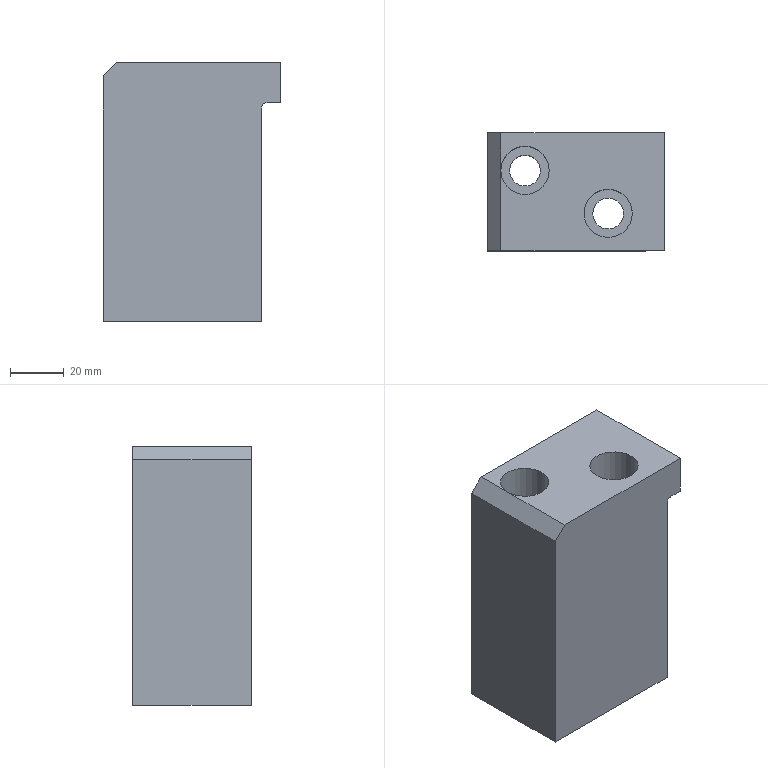Part | NX | features solid 2 | 1 solid | 16 faces | box 66 x 44 x 96.5 mm | volume 210931 mm3 | plane 11 | cylinder 5 | commonest cylinder face diameters 11.5 x2 18 x2 4 x1
STEP:
#1=CARTESIAN_POINT('',(1496.,74.,-16.5));
#2=VERTEX_POINT('',#1);
#3=CARTESIAN_POINT('',(1487.,74.,-16.5));
#4=DIRECTION('',(0.,0.,-1.));
#5=DIRECTION('',(1.,0.,0.));
#6=AXIS2_PLACEMENT_3D('',#3,#4,#5);
#7=CIRCLE('',#6,9.);
#8=EDGE_CURVE('',#2,#2,#7,.T.);
#9=ORIENTED_EDGE('',*,*,#8,.T.);
#10=EDGE_LOOP('',(#9));
#11=FACE_BOUND('',#10,.T.);
#12=CARTESIAN_POINT('',(1508.,104.,-16.5));
#13=VERTEX_POINT('',#12);
#14=CARTESIAN_POINT('',(1447.,104.,-16.5));
#15=VERTEX_POINT('',#14);
#16=CARTESIAN_POINT('',(1471.,104.,-16.5));
#17=DIRECTION('',(-1.,0.,0.));
#18=VECTOR('',#17,1000.);
#19=LINE('',#16,#18);
#20=EDGE_CURVE('',#13,#15,#19,.T.);
#21=ORIENTED_EDGE('',*,*,#20,.T.);
#22=CARTESIAN_POINT('',(1447.,90.,-16.5));
#23=VERTEX_POINT('',#22);
#24=CARTESIAN_POINT('',(1447.,82.,-16.5));
#25=DIRECTION('',(0.,-1.,0.));
#26=VECTOR('',#25,1000.);
#27=LINE('',#24,#26);
#28=EDGE_CURVE('',#15,#23,#27,.T.);
#29=ORIENTED_EDGE('',*,*,#28,.T.);
#30=CARTESIAN_POINT('',(1456.,90.,-16.5));
#31=DIRECTION('',(0.,0.,-1.));
#32=DIRECTION('',(1.,0.,0.));
#33=AXIS2_PLACEMENT_3D('',#30,#31,#32);
#34=CIRCLE('',#33,9.);
#35=EDGE_CURVE('',#23,#23,#34,.T.);
#36=ORIENTED_EDGE('',*,*,#35,.T.);
#37=CARTESIAN_POINT('',(1447.,60.,-16.5));
#38=VERTEX_POINT('',#37);
#39=CARTESIAN_POINT('',(1447.,82.,-16.5));
#40=DIRECTION('',(0.,-1.,0.));
#41=VECTOR('',#40,1000.);
#42=LINE('',#39,#41);
#43=EDGE_CURVE('',#23,#38,#42,.T.);
#44=ORIENTED_EDGE('',*,*,#43,.T.);
#45=CARTESIAN_POINT('',(1508.,60.,-16.5));
#46=VERTEX_POINT('',#45);
#47=CARTESIAN_POINT('',(1471.,60.,-16.5));
#48=DIRECTION('',(1.,0.,0.));
#49=VECTOR('',#48,1000.);
#50=LINE('',#47,#49);
#51=EDGE_CURVE('',#38,#46,#50,.T.);
#52=ORIENTED_EDGE('',*,*,#51,.T.);
#53=CARTESIAN_POINT('',(1508.,82.,-16.5));
#54=DIRECTION('',(0.,1.,0.));
#55=VECTOR('',#54,1000.);
#56=LINE('',#53,#55);
#57=EDGE_CURVE('',#46,#13,#56,.T.);
#58=ORIENTED_EDGE('',*,*,#57,.T.);
#59=EDGE_LOOP('',(#21,#29,#36,#44,#52,#58));
#60=FACE_BOUND('',#59,.T.);
#61=CARTESIAN_POINT('',(1524.5,82.,-16.5));
#62=DIRECTION('',(0.,0.,1.));
#63=DIRECTION('',(-1.,0.,0.));
#64=AXIS2_PLACEMENT_3D('',#61,#62,#63);
#65=PLANE('',#64);
#66=ADVANCED_FACE('',(#11,#60),#65,.T.);
#67=CARTESIAN_POINT('',(1442.,104.,-113.));
#68=VERTEX_POINT('',#67);
#69=CARTESIAN_POINT('',(1442.,104.,-21.5));
#70=VERTEX_POINT('',#69);
#71=CARTESIAN_POINT('',(1442.,104.,-88.5));
#72=DIRECTION('',(0.,0.,1.));
#73=VECTOR('',#72,1000.);
#74=LINE('',#71,#73);
#75=EDGE_CURVE('',#68,#70,#74,.T.);
#76=ORIENTED_EDGE('',*,*,#75,.T.);
#77=CARTESIAN_POINT('',(1404.75,104.,-58.75));
#78=DIRECTION('',(0.7071,0.,0.7071));
#79=VECTOR('',#78,1000.);
#80=LINE('',#77,#79);
#81=EDGE_CURVE('',#70,#15,#80,.T.);
#82=ORIENTED_EDGE('',*,*,#81,.T.);
#83=ORIENTED_EDGE('',*,*,#20,.F.);
#84=CARTESIAN_POINT('',(1508.,104.,-31.5));
#85=VERTEX_POINT('',#84);
#86=CARTESIAN_POINT('',(1508.,104.,-125.));
#87=DIRECTION('',(0.,0.,1.));
#88=VECTOR('',#87,1000.);
#89=LINE('',#86,#88);
#90=EDGE_CURVE('',#85,#13,#89,.T.);
#91=ORIENTED_EDGE('',*,*,#90,.F.);
#92=CARTESIAN_POINT('',(1503.,104.,-31.5));
#93=VERTEX_POINT('',#92);
#94=CARTESIAN_POINT('',(1471.,104.,-31.5));
#95=DIRECTION('',(-1.,0.,0.));
#96=VECTOR('',#95,1000.);
#97=LINE('',#94,#96);
#98=EDGE_CURVE('',#85,#93,#97,.T.);
#99=ORIENTED_EDGE('',*,*,#98,.T.);
#100=CARTESIAN_POINT('',(1501.,104.,-33.5));
#101=VERTEX_POINT('',#100);
#102=CARTESIAN_POINT('',(1503.,104.,-33.5));
#103=DIRECTION('',(0.,1.,0.));
#104=DIRECTION('',(0.,0.,-1.));
#105=AXIS2_PLACEMENT_3D('',#102,#103,#104);
#106=CIRCLE('',#105,2.);
#107=EDGE_CURVE('',#101,#93,#106,.T.);
#108=ORIENTED_EDGE('',*,*,#107,.F.);
#109=CARTESIAN_POINT('',(1501.,104.,-113.));
#110=VERTEX_POINT('',#109);
#111=CARTESIAN_POINT('',(1501.,104.,-125.));
#112=DIRECTION('',(0.,0.,1.));
#113=VECTOR('',#112,1000.);
#114=LINE('',#111,#113);
#115=EDGE_CURVE('',#110,#101,#114,.T.);
#116=ORIENTED_EDGE('',*,*,#115,.F.);
#117=CARTESIAN_POINT('',(1471.,104.,-113.));
#118=DIRECTION('',(1.,0.,0.));
#119=VECTOR('',#118,1000.);
#120=LINE('',#117,#119);
#121=EDGE_CURVE('',#68,#110,#120,.T.);
#122=ORIENTED_EDGE('',*,*,#121,.F.);
#123=EDGE_LOOP('',(#76,#82,#83,#91,#99,#108,#116,#122));
#124=FACE_BOUND('',#123,.T.);
#125=CARTESIAN_POINT('',(1471.,104.,-125.));
#126=DIRECTION('',(0.,1.,0.));
#127=DIRECTION('',(0.,0.,1.));
#128=AXIS2_PLACEMENT_3D('',#125,#126,#127);
#129=PLANE('',#128);
#130=ADVANCED_FACE('',(#124),#129,.T.);
#131=CARTESIAN_POINT('',(1442.,60.,-113.));
#132=VERTEX_POINT('',#131);
#133=CARTESIAN_POINT('',(1442.,60.,-21.5));
#134=VERTEX_POINT('',#133);
#135=CARTESIAN_POINT('',(1442.,60.,-125.));
#136=DIRECTION('',(0.,0.,1.));
#137=VECTOR('',#136,1000.);
#138=LINE('',#135,#137);
#139=EDGE_CURVE('',#132,#134,#138,.T.);
#140=ORIENTED_EDGE('',*,*,#139,.T.);
#141=CARTESIAN_POINT('',(1442.,82.,-21.5));
#142=DIRECTION('',(0.,1.,0.));
#143=VECTOR('',#142,1000.);
#144=LINE('',#141,#143);
#145=EDGE_CURVE('',#134,#70,#144,.T.);
#146=ORIENTED_EDGE('',*,*,#145,.T.);
#147=ORIENTED_EDGE('',*,*,#75,.F.);
#148=CARTESIAN_POINT('',(1442.,82.,-113.));
#149=DIRECTION('',(0.,1.,0.));
#150=VECTOR('',#149,1000.);
#151=LINE('',#148,#150);
#152=EDGE_CURVE('',#132,#68,#151,.T.);
#153=ORIENTED_EDGE('',*,*,#152,.F.);
#154=EDGE_LOOP('',(#140,#146,#147,#153));
#155=FACE_BOUND('',#154,.T.);
#156=CARTESIAN_POINT('',(1442.,82.,-88.5));
#157=DIRECTION('',(-1.,0.,0.));
#158=DIRECTION('',(0.,0.,-1.));
#159=AXIS2_PLACEMENT_3D('',#156,#157,#158);
#160=PLANE('',#159);
#161=ADVANCED_FACE('',(#155),#160,.T.);
#162=ORIENTED_EDGE('',*,*,#51,.F.);
#163=CARTESIAN_POINT('',(1404.75,60.,-58.75));
#164=DIRECTION('',(-0.7071,0.,-0.7071));
#165=VECTOR('',#164,1000.);
#166=LINE('',#163,#165);
#167=EDGE_CURVE('',#38,#134,#166,.T.);
#168=ORIENTED_EDGE('',*,*,#167,.T.);
#169=ORIENTED_EDGE('',*,*,#139,.F.);
#170=CARTESIAN_POINT('',(1501.,60.,-113.));
#171=VERTEX_POINT('',#170);
#172=CARTESIAN_POINT('',(1471.,60.,-113.));
#173=DIRECTION('',(-1.,0.,0.));
#174=VECTOR('',#173,1000.);
#175=LINE('',#172,#174);
#176=EDGE_CURVE('',#171,#132,#175,.T.);
#177=ORIENTED_EDGE('',*,*,#176,.F.);
#178=CARTESIAN_POINT('',(1501.,60.,-33.5));
#179=VERTEX_POINT('',#178);
#180=CARTESIAN_POINT('',(1501.,60.,-125.));
#181=DIRECTION('',(0.,0.,1.));
#182=VECTOR('',#181,1000.);
#183=LINE('',#180,#182);
#184=EDGE_CURVE('',#171,#179,#183,.T.);
#185=ORIENTED_EDGE('',*,*,#184,.T.);
#186=CARTESIAN_POINT('',(1503.,60.,-31.5));
#187=VERTEX_POINT('',#186);
#188=CARTESIAN_POINT('',(1503.,60.,-33.5));
#189=DIRECTION('',(0.,-1.,0.));
#190=DIRECTION('',(0.,0.,1.));
#191=AXIS2_PLACEMENT_3D('',#188,#189,#190);
#192=CIRCLE('',#191,2.);
#193=EDGE_CURVE('',#187,#179,#192,.T.);
#194=ORIENTED_EDGE('',*,*,#193,.F.);
#195=CARTESIAN_POINT('',(1508.,60.,-31.5));
#196=VERTEX_POINT('',#195);
#197=CARTESIAN_POINT('',(1471.,60.,-31.5));
#198=DIRECTION('',(-1.,0.,0.));
#199=VECTOR('',#198,1000.);
#200=LINE('',#197,#199);
#201=EDGE_CURVE('',#196,#187,#200,.T.);
#202=ORIENTED_EDGE('',*,*,#201,.F.);
#203=CARTESIAN_POINT('',(1508.,60.,-125.));
#204=DIRECTION('',(0.,0.,1.));
#205=VECTOR('',#204,1000.);
#206=LINE('',#203,#205);
#207=EDGE_CURVE('',#196,#46,#206,.T.);
#208=ORIENTED_EDGE('',*,*,#207,.T.);
#209=EDGE_LOOP('',(#162,#168,#169,#177,#185,#194,#202,#208));
#210=FACE_BOUND('',#209,.T.);
#211=CARTESIAN_POINT('',(1471.,60.,-125.));
#212=DIRECTION('',(0.,-1.,0.));
#213=DIRECTION('',(0.,0.,-1.));
#214=AXIS2_PLACEMENT_3D('',#211,#212,#213);
#215=PLANE('',#214);
#216=ADVANCED_FACE('',(#210),#215,.T.);
#217=CARTESIAN_POINT('',(1508.,82.,-31.5));
#218=DIRECTION('',(0.,1.,0.));
#219=VECTOR('',#218,1000.);
#220=LINE('',#217,#219);
#221=EDGE_CURVE('',#196,#85,#220,.T.);
#222=ORIENTED_EDGE('',*,*,#221,.T.);
#223=ORIENTED_EDGE('',*,*,#90,.T.);
#224=ORIENTED_EDGE('',*,*,#57,.F.);
#225=ORIENTED_EDGE('',*,*,#207,.F.);
#226=EDGE_LOOP('',(#222,#223,#224,#225));
#227=FACE_BOUND('',#226,.T.);
#228=CARTESIAN_POINT('',(1508.,82.,-125.));
#229=DIRECTION('',(1.,0.,0.));
#230=DIRECTION('',(0.,0.,1.));
#231=AXIS2_PLACEMENT_3D('',#228,#229,#230);
#232=PLANE('',#231);
#233=ADVANCED_FACE('',(#227),#232,.T.);
#234=ORIENTED_EDGE('',*,*,#98,.F.);
#235=ORIENTED_EDGE('',*,*,#221,.F.);
#236=ORIENTED_EDGE('',*,*,#201,.T.);
#237=CARTESIAN_POINT('',(1503.,82.,-31.5));
#238=DIRECTION('',(0.,-1.,0.));
#239=VECTOR('',#238,1000.);
#240=LINE('',#237,#239);
#241=EDGE_CURVE('',#93,#187,#240,.T.);
#242=ORIENTED_EDGE('',*,*,#241,.F.);
#243=EDGE_LOOP('',(#234,#235,#236,#242));
#244=FACE_BOUND('',#243,.T.);
#245=CARTESIAN_POINT('',(1471.5,82.,-31.5));
#246=DIRECTION('',(0.,0.,1.));
#247=DIRECTION('',(-1.,0.,0.));
#248=AXIS2_PLACEMENT_3D('',#245,#246,#247);
#249=PLANE('',#248);
#250=ADVANCED_FACE('',(#244),#249,.F.);
#251=CARTESIAN_POINT('',(1450.25,90.,-113.));
#252=VERTEX_POINT('',#251);
#253=CARTESIAN_POINT('',(1456.,90.,-113.));
#254=DIRECTION('',(0.,0.,1.));
#255=DIRECTION('',(-1.,0.,0.));
#256=AXIS2_PLACEMENT_3D('',#253,#254,#255);
#257=CIRCLE('',#256,5.75);
#258=EDGE_CURVE('',#252,#252,#257,.T.);
#259=ORIENTED_EDGE('',*,*,#258,.T.);
#260=EDGE_LOOP('',(#259));
#261=FACE_BOUND('',#260,.T.);
#262=CARTESIAN_POINT('',(1481.25,74.,-113.));
#263=VERTEX_POINT('',#262);
#264=CARTESIAN_POINT('',(1487.,74.,-113.));
#265=DIRECTION('',(0.,0.,1.));
#266=DIRECTION('',(-1.,0.,0.));
#267=AXIS2_PLACEMENT_3D('',#264,#265,#266);
#268=CIRCLE('',#267,5.75);
#269=EDGE_CURVE('',#263,#263,#268,.T.);
#270=ORIENTED_EDGE('',*,*,#269,.T.);
#271=EDGE_LOOP('',(#270));
#272=FACE_BOUND('',#271,.T.);
#273=CARTESIAN_POINT('',(1501.,82.,-113.));
#274=DIRECTION('',(0.,-1.,0.));
#275=VECTOR('',#274,1000.);
#276=LINE('',#273,#275);
#277=EDGE_CURVE('',#110,#171,#276,.T.);
#278=ORIENTED_EDGE('',*,*,#277,.T.);
#279=ORIENTED_EDGE('',*,*,#176,.T.);
#280=ORIENTED_EDGE('',*,*,#152,.T.);
#281=ORIENTED_EDGE('',*,*,#121,.T.);
#282=EDGE_LOOP('',(#278,#279,#280,#281));
#283=FACE_BOUND('',#282,.T.);
#284=CARTESIAN_POINT('',(1920.,-43.,-113.));
#285=DIRECTION('',(0.,0.,-1.));
#286=DIRECTION('',(1.,0.,0.));
#287=AXIS2_PLACEMENT_3D('',#284,#285,#286);
#288=PLANE('',#287);
#289=ADVANCED_FACE('',(#261,#272,#283),#288,.T.);
#290=ORIENTED_EDGE('',*,*,#184,.F.);
#291=ORIENTED_EDGE('',*,*,#277,.F.);
#292=ORIENTED_EDGE('',*,*,#115,.T.);
#293=CARTESIAN_POINT('',(1501.,82.,-33.5));
#294=DIRECTION('',(0.,1.,0.));
#295=VECTOR('',#294,1000.);
#296=LINE('',#293,#295);
#297=EDGE_CURVE('',#179,#101,#296,.T.);
#298=ORIENTED_EDGE('',*,*,#297,.F.);
#299=EDGE_LOOP('',(#290,#291,#292,#298));
#300=FACE_BOUND('',#299,.T.);
#301=CARTESIAN_POINT('',(1501.,82.,-125.));
#302=DIRECTION('',(1.,0.,0.));
#303=DIRECTION('',(0.,0.,1.));
#304=AXIS2_PLACEMENT_3D('',#301,#302,#303);
#305=PLANE('',#304);
#306=ADVANCED_FACE('',(#300),#305,.T.);
#307=ORIENTED_EDGE('',*,*,#269,.F.);
#308=EDGE_LOOP('',(#307));
#309=FACE_BOUND('',#308,.T.);
#310=CARTESIAN_POINT('',(1481.25,74.,-95.));
#311=VERTEX_POINT('',#310);
#312=CARTESIAN_POINT('',(1487.,74.,-95.));
#313=DIRECTION('',(0.,0.,1.));
#314=DIRECTION('',(-1.,0.,0.));
#315=AXIS2_PLACEMENT_3D('',#312,#313,#314);
#316=CIRCLE('',#315,5.75);
#317=EDGE_CURVE('',#311,#311,#316,.T.);
#318=ORIENTED_EDGE('',*,*,#317,.T.);
#319=EDGE_LOOP('',(#318));
#320=FACE_BOUND('',#319,.T.);
#321=CARTESIAN_POINT('',(1487.,74.,-29.5));
#322=DIRECTION('',(0.,0.,-1.));
#323=DIRECTION('',(-1.,0.,0.));
#324=AXIS2_PLACEMENT_3D('',#321,#322,#323);
#325=CYLINDRICAL_SURFACE('',#324,5.75);
#326=ADVANCED_FACE('',(#309,#320),#325,.F.);
#327=ORIENTED_EDGE('',*,*,#317,.F.);
#328=EDGE_LOOP('',(#327));
#329=FACE_BOUND('',#328,.T.);
#330=CARTESIAN_POINT('',(1496.,74.,-95.));
#331=VERTEX_POINT('',#330);
#332=CARTESIAN_POINT('',(1487.,74.,-95.));
#333=DIRECTION('',(0.,0.,1.));
#334=DIRECTION('',(1.,0.,0.));
#335=AXIS2_PLACEMENT_3D('',#332,#333,#334);
#336=CIRCLE('',#335,9.);
#337=EDGE_CURVE('',#331,#331,#336,.T.);
#338=ORIENTED_EDGE('',*,*,#337,.T.);
#339=EDGE_LOOP('',(#338));
#340=FACE_BOUND('',#339,.T.);
#341=CARTESIAN_POINT('',(1487.,74.,-95.));
#342=DIRECTION('',(0.,0.,-1.));
#343=DIRECTION('',(1.,0.,0.));
#344=AXIS2_PLACEMENT_3D('',#341,#342,#343);
#345=PLANE('',#344);
#346=ADVANCED_FACE('',(#329,#340),#345,.F.);
#347=ORIENTED_EDGE('',*,*,#337,.F.);
#348=EDGE_LOOP('',(#347));
#349=FACE_BOUND('',#348,.T.);
#350=ORIENTED_EDGE('',*,*,#8,.F.);
#351=EDGE_LOOP('',(#350));
#352=FACE_BOUND('',#351,.T.);
#353=CARTESIAN_POINT('',(1487.,74.,-31.5));
#354=DIRECTION('',(0.,0.,-1.));
#355=DIRECTION('',(-1.,0.,0.));
#356=AXIS2_PLACEMENT_3D('',#353,#354,#355);
#357=CYLINDRICAL_SURFACE('',#356,9.);
#358=ADVANCED_FACE('',(#349,#352),#357,.F.);
#359=ORIENTED_EDGE('',*,*,#258,.F.);
#360=EDGE_LOOP('',(#359));
#361=FACE_BOUND('',#360,.T.);
#362=CARTESIAN_POINT('',(1450.25,90.,-95.));
#363=VERTEX_POINT('',#362);
#364=CARTESIAN_POINT('',(1456.,90.,-95.));
#365=DIRECTION('',(0.,0.,1.));
#366=DIRECTION('',(-1.,0.,0.));
#367=AXIS2_PLACEMENT_3D('',#364,#365,#366);
#368=CIRCLE('',#367,5.75);
#369=EDGE_CURVE('',#363,#363,#368,.T.);
#370=ORIENTED_EDGE('',*,*,#369,.T.);
#371=EDGE_LOOP('',(#370));
#372=FACE_BOUND('',#371,.T.);
#373=CARTESIAN_POINT('',(1456.,90.,-29.5));
#374=DIRECTION('',(0.,0.,-1.));
#375=DIRECTION('',(-1.,0.,0.));
#376=AXIS2_PLACEMENT_3D('',#373,#374,#375);
#377=CYLINDRICAL_SURFACE('',#376,5.75);
#378=ADVANCED_FACE('',(#361,#372),#377,.F.);
#379=ORIENTED_EDGE('',*,*,#369,.F.);
#380=EDGE_LOOP('',(#379));
#381=FACE_BOUND('',#380,.T.);
#382=CARTESIAN_POINT('',(1465.,90.,-95.));
#383=VERTEX_POINT('',#382);
#384=CARTESIAN_POINT('',(1456.,90.,-95.));
#385=DIRECTION('',(0.,0.,1.));
#386=DIRECTION('',(1.,0.,0.));
#387=AXIS2_PLACEMENT_3D('',#384,#385,#386);
#388=CIRCLE('',#387,9.);
#389=EDGE_CURVE('',#383,#383,#388,.T.);
#390=ORIENTED_EDGE('',*,*,#389,.T.);
#391=EDGE_LOOP('',(#390));
#392=FACE_BOUND('',#391,.T.);
#393=CARTESIAN_POINT('',(1456.,90.,-95.));
#394=DIRECTION('',(0.,0.,-1.));
#395=DIRECTION('',(1.,0.,0.));
#396=AXIS2_PLACEMENT_3D('',#393,#394,#395);
#397=PLANE('',#396);
#398=ADVANCED_FACE('',(#381,#392),#397,.F.);
#399=ORIENTED_EDGE('',*,*,#389,.F.);
#400=EDGE_LOOP('',(#399));
#401=FACE_BOUND('',#400,.T.);
#402=ORIENTED_EDGE('',*,*,#35,.F.);
#403=EDGE_LOOP('',(#402));
#404=FACE_BOUND('',#403,.T.);
#405=CARTESIAN_POINT('',(1456.,90.,-31.5));
#406=DIRECTION('',(0.,0.,-1.));
#407=DIRECTION('',(-1.,0.,0.));
#408=AXIS2_PLACEMENT_3D('',#405,#406,#407);
#409=CYLINDRICAL_SURFACE('',#408,9.);
#410=ADVANCED_FACE('',(#401,#404),#409,.F.);
#411=ORIENTED_EDGE('',*,*,#107,.T.);
#412=ORIENTED_EDGE('',*,*,#241,.T.);
#413=ORIENTED_EDGE('',*,*,#193,.T.);
#414=ORIENTED_EDGE('',*,*,#297,.T.);
#415=EDGE_LOOP('',(#411,#412,#413,#414));
#416=FACE_BOUND('',#415,.T.);
#417=CARTESIAN_POINT('',(1503.,82.,-33.5));
#418=DIRECTION('',(0.,-1.,0.));
#419=DIRECTION('',(0.,0.,-1.));
#420=AXIS2_PLACEMENT_3D('',#417,#418,#419);
#421=CYLINDRICAL_SURFACE('',#420,2.);
#422=ADVANCED_FACE('',(#416),#421,.F.);
#423=ORIENTED_EDGE('',*,*,#81,.F.);
#424=ORIENTED_EDGE('',*,*,#145,.F.);
#425=ORIENTED_EDGE('',*,*,#167,.F.);
#426=ORIENTED_EDGE('',*,*,#43,.F.);
#427=ORIENTED_EDGE('',*,*,#28,.F.);
#428=EDGE_LOOP('',(#423,#424,#425,#426,#427));
#429=FACE_BOUND('',#428,.T.);
#430=CARTESIAN_POINT('',(1447.,82.,-16.5));
#431=DIRECTION('',(0.7071,0.,-0.7071));
#432=DIRECTION('',(0.,1.,0.));
#433=AXIS2_PLACEMENT_3D('',#430,#431,#432);
#434=PLANE('',#433);
#435=ADVANCED_FACE('',(#429),#434,.F.);
#436=CLOSED_SHELL('',(#66,#130,#161,#216,#233,#250,#289,#306,#326,#346,#358,#378,#398,#410,#422,#435));
#437=MANIFOLD_SOLID_BREP('',#436);
#438=(LENGTH_UNIT()NAMED_UNIT(*)SI_UNIT(.MILLI.,.METRE.));
#439=UNCERTAINTY_MEASURE_WITH_UNIT(LENGTH_MEASURE(0.00001),#438,'','');
#440=(NAMED_UNIT(*)PLANE_ANGLE_UNIT()SI_UNIT($,.RADIAN.));
#441=(NAMED_UNIT(*)SI_UNIT($,.STERADIAN.)SOLID_ANGLE_UNIT());
#442=(GEOMETRIC_REPRESENTATION_CONTEXT(3)GLOBAL_UNCERTAINTY_ASSIGNED_CONTEXT((#439))GLOBAL_UNIT_ASSIGNED_CONTEXT((#438,#440,#441))REPRESENTATION_CONTEXT('',''));
#443=ADVANCED_BREP_SHAPE_REPRESENTATION('',(#437),#442);